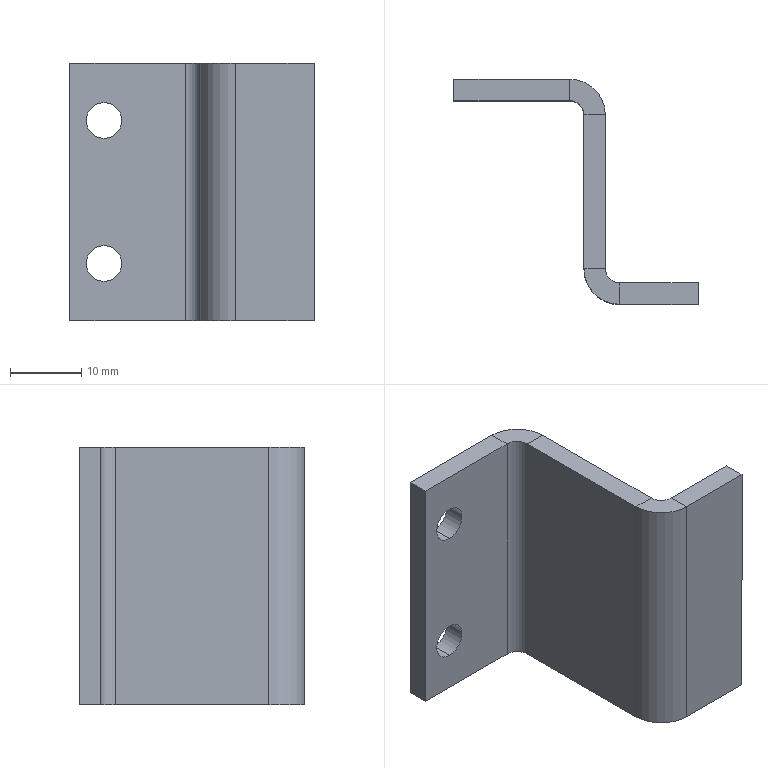Part | SolidWorks | features EdgeFlange 2, FlatPattern 1, HoleWzd 1, SMBaseFlange 1, SheetMetal 1 | 1 solid | 26 faces | box 34.18 x 31.5 x 36 mm | volume 6327 mm3 | plane 18 | cylinder 8 | commonest cylinder face diameters 5 x4 4 x2 10 x2
STEP:
#1=CARTESIAN_POINT('',(-21.41,25.5,-12.5));
#2=VERTEX_POINT('',#1);
#3=CARTESIAN_POINT('',(-21.41,25.5,-7.5));
#4=VERTEX_POINT('',#3);
#5=CARTESIAN_POINT('',(-21.41,25.5,-10.));
#6=DIRECTION('',(0.,1.,0.));
#7=DIRECTION('',(0.,0.,1.));
#8=AXIS2_PLACEMENT_3D('',#5,#6,#7);
#9=CIRCLE('',#8,2.5);
#10=EDGE_CURVE('',#2,#4,#9,.T.);
#11=ORIENTED_EDGE('',*,*,#10,.F.);
#12=CARTESIAN_POINT('',(-21.41,28.5,-12.5));
#13=VERTEX_POINT('',#12);
#14=CARTESIAN_POINT('',(-21.41,28.5,-12.5));
#15=DIRECTION('',(0.,1.,0.));
#16=VECTOR('',#15,1000.);
#17=LINE('',#14,#16);
#18=EDGE_CURVE('',#2,#13,#17,.T.);
#19=ORIENTED_EDGE('',*,*,#18,.T.);
#20=CARTESIAN_POINT('',(-21.41,28.5,-7.5));
#21=VERTEX_POINT('',#20);
#22=CARTESIAN_POINT('',(-21.41,28.5,-10.));
#23=DIRECTION('',(0.,1.,0.));
#24=DIRECTION('',(0.,0.,1.));
#25=AXIS2_PLACEMENT_3D('',#22,#23,#24);
#26=CIRCLE('',#25,2.5);
#27=EDGE_CURVE('',#13,#21,#26,.T.);
#28=ORIENTED_EDGE('',*,*,#27,.T.);
#29=CARTESIAN_POINT('',(-21.41,28.5,-7.5));
#30=DIRECTION('',(0.,1.,0.));
#31=VECTOR('',#30,1000.);
#32=LINE('',#29,#31);
#33=EDGE_CURVE('',#4,#21,#32,.T.);
#34=ORIENTED_EDGE('',*,*,#33,.F.);
#35=EDGE_LOOP('',(#11,#19,#28,#34));
#36=FACE_OUTER_BOUND('',#35,.T.);
#37=CARTESIAN_POINT('',(-21.41,28.5,-10.));
#38=DIRECTION('',(0.,1.,0.));
#39=DIRECTION('',(0.,0.,1.));
#40=AXIS2_PLACEMENT_3D('',#37,#38,#39);
#41=CYLINDRICAL_SURFACE('',#40,2.5);
#42=ADVANCED_FACE('',(#36),#41,.F.);
#43=CARTESIAN_POINT('',(-21.41,25.5,7.5));
#44=VERTEX_POINT('',#43);
#45=CARTESIAN_POINT('',(-21.41,25.5,12.5));
#46=VERTEX_POINT('',#45);
#47=CARTESIAN_POINT('',(-21.41,25.5,10.));
#48=DIRECTION('',(0.,1.,0.));
#49=DIRECTION('',(0.,0.,1.));
#50=AXIS2_PLACEMENT_3D('',#47,#48,#49);
#51=CIRCLE('',#50,2.5);
#52=EDGE_CURVE('',#44,#46,#51,.T.);
#53=ORIENTED_EDGE('',*,*,#52,.F.);
#54=CARTESIAN_POINT('',(-21.41,28.5,7.5));
#55=VERTEX_POINT('',#54);
#56=CARTESIAN_POINT('',(-21.41,28.5,7.5));
#57=DIRECTION('',(0.,1.,0.));
#58=VECTOR('',#57,1000.);
#59=LINE('',#56,#58);
#60=EDGE_CURVE('',#44,#55,#59,.T.);
#61=ORIENTED_EDGE('',*,*,#60,.T.);
#62=CARTESIAN_POINT('',(-21.41,28.5,12.5));
#63=VERTEX_POINT('',#62);
#64=CARTESIAN_POINT('',(-21.41,28.5,10.));
#65=DIRECTION('',(0.,1.,0.));
#66=DIRECTION('',(0.,0.,1.));
#67=AXIS2_PLACEMENT_3D('',#64,#65,#66);
#68=CIRCLE('',#67,2.5);
#69=EDGE_CURVE('',#55,#63,#68,.T.);
#70=ORIENTED_EDGE('',*,*,#69,.T.);
#71=CARTESIAN_POINT('',(-21.41,28.5,12.5));
#72=DIRECTION('',(0.,1.,0.));
#73=VECTOR('',#72,1000.);
#74=LINE('',#71,#73);
#75=EDGE_CURVE('',#46,#63,#74,.T.);
#76=ORIENTED_EDGE('',*,*,#75,.F.);
#77=EDGE_LOOP('',(#53,#61,#70,#76));
#78=FACE_OUTER_BOUND('',#77,.T.);
#79=CARTESIAN_POINT('',(-21.41,28.5,10.));
#80=DIRECTION('',(0.,1.,0.));
#81=DIRECTION('',(0.,0.,1.));
#82=AXIS2_PLACEMENT_3D('',#79,#80,#81);
#83=CYLINDRICAL_SURFACE('',#82,2.5);
#84=ADVANCED_FACE('',(#78),#83,.F.);
#85=CARTESIAN_POINT('',(-7.99,2.,-18.));
#86=VERTEX_POINT('',#85);
#87=CARTESIAN_POINT('',(-7.99,23.5,-18.));
#88=VERTEX_POINT('',#87);
#89=CARTESIAN_POINT('',(-7.99,28.5,-18.));
#90=DIRECTION('',(0.,1.,0.));
#91=VECTOR('',#90,1000.);
#92=LINE('',#89,#91);
#93=EDGE_CURVE('',#86,#88,#92,.T.);
#94=ORIENTED_EDGE('',*,*,#93,.T.);
#95=CARTESIAN_POINT('',(-4.99,23.5,-18.));
#96=VERTEX_POINT('',#95);
#97=CARTESIAN_POINT('',(-7.99,23.5,-18.));
#98=DIRECTION('',(1.,0.,0.));
#99=VECTOR('',#98,1000.);
#100=LINE('',#97,#99);
#101=EDGE_CURVE('',#88,#96,#100,.T.);
#102=ORIENTED_EDGE('',*,*,#101,.T.);
#103=CARTESIAN_POINT('',(-4.99,2.,-18.));
#104=VERTEX_POINT('',#103);
#105=CARTESIAN_POINT('',(-4.99,0.,-18.));
#106=DIRECTION('',(0.,1.,0.));
#107=VECTOR('',#106,1000.);
#108=LINE('',#105,#107);
#109=EDGE_CURVE('',#104,#96,#108,.T.);
#110=ORIENTED_EDGE('',*,*,#109,.F.);
#111=CARTESIAN_POINT('',(-7.99,2.,-18.));
#112=DIRECTION('',(-1.,0.,0.));
#113=VECTOR('',#112,1000.);
#114=LINE('',#111,#113);
#115=EDGE_CURVE('',#104,#86,#114,.T.);
#116=ORIENTED_EDGE('',*,*,#115,.T.);
#117=EDGE_LOOP('',(#94,#102,#110,#116));
#118=FACE_OUTER_BOUND('',#117,.T.);
#119=CARTESIAN_POINT('',(-7.99,28.5,-18.));
#120=DIRECTION('',(0.,0.,-1.));
#121=DIRECTION('',(-1.,0.,0.));
#122=AXIS2_PLACEMENT_3D('',#119,#120,#121);
#123=PLANE('',#122);
#124=ADVANCED_FACE('',(#118),#123,.T.);
#125=CARTESIAN_POINT('',(-7.99,23.5,18.));
#126=VERTEX_POINT('',#125);
#127=CARTESIAN_POINT('',(-7.99,2.,18.));
#128=VERTEX_POINT('',#127);
#129=CARTESIAN_POINT('',(-7.99,0.,18.));
#130=DIRECTION('',(0.,-1.,0.));
#131=VECTOR('',#130,1000.);
#132=LINE('',#129,#131);
#133=EDGE_CURVE('',#126,#128,#132,.T.);
#134=ORIENTED_EDGE('',*,*,#133,.F.);
#135=CARTESIAN_POINT('',(-7.99,23.5,-18.));
#136=DIRECTION('',(0.,0.,1.));
#137=VECTOR('',#136,1000.);
#138=LINE('',#135,#137);
#139=EDGE_CURVE('',#88,#126,#138,.T.);
#140=ORIENTED_EDGE('',*,*,#139,.F.);
#141=ORIENTED_EDGE('',*,*,#93,.F.);
#142=CARTESIAN_POINT('',(-7.99,2.,0.));
#143=DIRECTION('',(0.,0.,1.));
#144=VECTOR('',#143,1000.);
#145=LINE('',#142,#144);
#146=EDGE_CURVE('',#86,#128,#145,.T.);
#147=ORIENTED_EDGE('',*,*,#146,.T.);
#148=EDGE_LOOP('',(#134,#140,#141,#147));
#149=FACE_OUTER_BOUND('',#148,.T.);
#150=CARTESIAN_POINT('',(-7.99,0.,0.));
#151=DIRECTION('',(-1.,0.,0.));
#152=DIRECTION('',(0.,-1.,0.));
#153=AXIS2_PLACEMENT_3D('',#150,#151,#152);
#154=PLANE('',#153);
#155=ADVANCED_FACE('',(#149),#154,.T.);
#156=CARTESIAN_POINT('',(-4.99,23.5,18.));
#157=VERTEX_POINT('',#156);
#158=CARTESIAN_POINT('',(-4.99,23.5,-18.));
#159=DIRECTION('',(0.,0.,1.));
#160=VECTOR('',#159,1000.);
#161=LINE('',#158,#160);
#162=EDGE_CURVE('',#96,#157,#161,.T.);
#163=ORIENTED_EDGE('',*,*,#162,.T.);
#164=CARTESIAN_POINT('',(-4.99,2.,18.));
#165=VERTEX_POINT('',#164);
#166=CARTESIAN_POINT('',(-4.99,0.,18.));
#167=DIRECTION('',(0.,-1.,0.));
#168=VECTOR('',#167,1000.);
#169=LINE('',#166,#168);
#170=EDGE_CURVE('',#157,#165,#169,.T.);
#171=ORIENTED_EDGE('',*,*,#170,.T.);
#172=CARTESIAN_POINT('',(-4.99,2.,-18.));
#173=DIRECTION('',(0.,0.,1.));
#174=VECTOR('',#173,1000.);
#175=LINE('',#172,#174);
#176=EDGE_CURVE('',#104,#165,#175,.T.);
#177=ORIENTED_EDGE('',*,*,#176,.F.);
#178=ORIENTED_EDGE('',*,*,#109,.T.);
#179=EDGE_LOOP('',(#163,#171,#177,#178));
#180=FACE_OUTER_BOUND('',#179,.T.);
#181=CARTESIAN_POINT('',(-4.99,0.,0.));
#182=DIRECTION('',(-1.,0.,0.));
#183=DIRECTION('',(0.,-1.,0.));
#184=AXIS2_PLACEMENT_3D('',#181,#182,#183);
#185=PLANE('',#184);
#186=ADVANCED_FACE('',(#180),#185,.F.);
#187=CARTESIAN_POINT('',(-2.99,0.,18.));
#188=VERTEX_POINT('',#187);
#189=CARTESIAN_POINT('',(7.99,0.,18.));
#190=VERTEX_POINT('',#189);
#191=CARTESIAN_POINT('',(-7.99,0.,18.));
#192=DIRECTION('',(1.,0.,0.));
#193=VECTOR('',#192,1000.);
#194=LINE('',#191,#193);
#195=EDGE_CURVE('',#188,#190,#194,.T.);
#196=ORIENTED_EDGE('',*,*,#195,.F.);
#197=CARTESIAN_POINT('',(-2.99,-3.,18.));
#198=VERTEX_POINT('',#197);
#199=CARTESIAN_POINT('',(-2.99,0.,18.));
#200=DIRECTION('',(0.,-1.,0.));
#201=VECTOR('',#200,1000.);
#202=LINE('',#199,#201);
#203=EDGE_CURVE('',#188,#198,#202,.T.);
#204=ORIENTED_EDGE('',*,*,#203,.T.);
#205=CARTESIAN_POINT('',(7.99,-3.,18.));
#206=VERTEX_POINT('',#205);
#207=CARTESIAN_POINT('',(-7.99,-3.,18.));
#208=DIRECTION('',(1.,0.,0.));
#209=VECTOR('',#208,1000.);
#210=LINE('',#207,#209);
#211=EDGE_CURVE('',#198,#206,#210,.T.);
#212=ORIENTED_EDGE('',*,*,#211,.T.);
#213=CARTESIAN_POINT('',(7.99,-3.,18.));
#214=DIRECTION('',(0.,1.,0.));
#215=VECTOR('',#214,1000.);
#216=LINE('',#213,#215);
#217=EDGE_CURVE('',#206,#190,#216,.T.);
#218=ORIENTED_EDGE('',*,*,#217,.T.);
#219=EDGE_LOOP('',(#196,#204,#212,#218));
#220=FACE_OUTER_BOUND('',#219,.T.);
#221=CARTESIAN_POINT('',(-7.99,-3.,18.));
#222=DIRECTION('',(0.,0.,1.));
#223=DIRECTION('',(1.,0.,0.));
#224=AXIS2_PLACEMENT_3D('',#221,#222,#223);
#225=PLANE('',#224);
#226=ADVANCED_FACE('',(#220),#225,.T.);
#227=CARTESIAN_POINT('',(-2.99,-3.,-18.));
#228=VERTEX_POINT('',#227);
#229=CARTESIAN_POINT('',(-2.99,-3.,18.));
#230=DIRECTION('',(0.,0.,-1.));
#231=VECTOR('',#230,1000.);
#232=LINE('',#229,#231);
#233=EDGE_CURVE('',#198,#228,#232,.T.);
#234=ORIENTED_EDGE('',*,*,#233,.T.);
#235=CARTESIAN_POINT('',(7.99,-3.,-18.));
#236=VERTEX_POINT('',#235);
#237=CARTESIAN_POINT('',(-7.99,-3.,-18.));
#238=DIRECTION('',(-1.,0.,0.));
#239=VECTOR('',#238,1000.);
#240=LINE('',#237,#239);
#241=EDGE_CURVE('',#236,#228,#240,.T.);
#242=ORIENTED_EDGE('',*,*,#241,.F.);
#243=CARTESIAN_POINT('',(7.99,-3.,-18.));
#244=DIRECTION('',(0.,0.,-1.));
#245=VECTOR('',#244,1000.);
#246=LINE('',#243,#245);
#247=EDGE_CURVE('',#206,#236,#246,.T.);
#248=ORIENTED_EDGE('',*,*,#247,.F.);
#249=ORIENTED_EDGE('',*,*,#211,.F.);
#250=EDGE_LOOP('',(#234,#242,#248,#249));
#251=FACE_OUTER_BOUND('',#250,.T.);
#252=CARTESIAN_POINT('',(0.,-3.,0.));
#253=DIRECTION('',(0.,1.,0.));
#254=DIRECTION('',(0.,0.,1.));
#255=AXIS2_PLACEMENT_3D('',#252,#253,#254);
#256=PLANE('',#255);
#257=ADVANCED_FACE('',(#251),#256,.F.);
#258=CARTESIAN_POINT('',(7.99,0.,-18.));
#259=VERTEX_POINT('',#258);
#260=CARTESIAN_POINT('',(-2.99,0.,-18.));
#261=VERTEX_POINT('',#260);
#262=CARTESIAN_POINT('',(-7.99,0.,-18.));
#263=DIRECTION('',(-1.,0.,0.));
#264=VECTOR('',#263,1000.);
#265=LINE('',#262,#264);
#266=EDGE_CURVE('',#259,#261,#265,.T.);
#267=ORIENTED_EDGE('',*,*,#266,.T.);
#268=CARTESIAN_POINT('',(-2.99,0.,18.));
#269=DIRECTION('',(0.,0.,-1.));
#270=VECTOR('',#269,1000.);
#271=LINE('',#268,#270);
#272=EDGE_CURVE('',#188,#261,#271,.T.);
#273=ORIENTED_EDGE('',*,*,#272,.F.);
#274=ORIENTED_EDGE('',*,*,#195,.T.);
#275=CARTESIAN_POINT('',(7.99,0.,-18.));
#276=DIRECTION('',(0.,0.,-1.));
#277=VECTOR('',#276,1000.);
#278=LINE('',#275,#277);
#279=EDGE_CURVE('',#190,#259,#278,.T.);
#280=ORIENTED_EDGE('',*,*,#279,.T.);
#281=EDGE_LOOP('',(#267,#273,#274,#280));
#282=FACE_OUTER_BOUND('',#281,.T.);
#283=CARTESIAN_POINT('',(0.,0.,0.));
#284=DIRECTION('',(0.,1.,0.));
#285=DIRECTION('',(0.,0.,1.));
#286=AXIS2_PLACEMENT_3D('',#283,#284,#285);
#287=PLANE('',#286);
#288=ADVANCED_FACE('',(#282),#287,.T.);
#289=ORIENTED_EDGE('',*,*,#279,.F.);
#290=ORIENTED_EDGE('',*,*,#217,.F.);
#291=ORIENTED_EDGE('',*,*,#247,.T.);
#292=CARTESIAN_POINT('',(7.99,-3.,-18.));
#293=DIRECTION('',(0.,1.,0.));
#294=VECTOR('',#293,1000.);
#295=LINE('',#292,#294);
#296=EDGE_CURVE('',#236,#259,#295,.T.);
#297=ORIENTED_EDGE('',*,*,#296,.T.);
#298=EDGE_LOOP('',(#289,#290,#291,#297));
#299=FACE_OUTER_BOUND('',#298,.T.);
#300=CARTESIAN_POINT('',(7.99,-3.,-18.));
#301=DIRECTION('',(1.,0.,0.));
#302=DIRECTION('',(0.,0.,-1.));
#303=AXIS2_PLACEMENT_3D('',#300,#301,#302);
#304=PLANE('',#303);
#305=ADVANCED_FACE('',(#299),#304,.T.);
#306=CARTESIAN_POINT('',(-2.99,0.,-18.));
#307=DIRECTION('',(0.,-1.,0.));
#308=VECTOR('',#307,1000.);
#309=LINE('',#306,#308);
#310=EDGE_CURVE('',#261,#228,#309,.T.);
#311=ORIENTED_EDGE('',*,*,#310,.F.);
#312=ORIENTED_EDGE('',*,*,#266,.F.);
#313=ORIENTED_EDGE('',*,*,#296,.F.);
#314=ORIENTED_EDGE('',*,*,#241,.T.);
#315=EDGE_LOOP('',(#311,#312,#313,#314));
#316=FACE_OUTER_BOUND('',#315,.T.);
#317=CARTESIAN_POINT('',(-7.99,-3.,-18.));
#318=DIRECTION('',(0.,0.,-1.));
#319=DIRECTION('',(-1.,0.,0.));
#320=AXIS2_PLACEMENT_3D('',#317,#318,#319);
#321=PLANE('',#320);
#322=ADVANCED_FACE('',(#316),#321,.T.);
#323=ORIENTED_EDGE('',*,*,#115,.F.);
#324=CARTESIAN_POINT('',(-2.99,2.,-18.));
#325=DIRECTION('',(0.,0.,-1.));
#326=DIRECTION('',(1.,0.,0.));
#327=AXIS2_PLACEMENT_3D('',#324,#325,#326);
#328=CIRCLE('',#327,2.);
#329=EDGE_CURVE('',#261,#104,#328,.T.);
#330=ORIENTED_EDGE('',*,*,#329,.F.);
#331=ORIENTED_EDGE('',*,*,#310,.T.);
#332=CARTESIAN_POINT('',(-2.99,2.,-18.));
#333=DIRECTION('',(0.,0.,-1.));
#334=DIRECTION('',(1.,0.,0.));
#335=AXIS2_PLACEMENT_3D('',#332,#333,#334);
#336=CIRCLE('',#335,5.);
#337=EDGE_CURVE('',#228,#86,#336,.T.);
#338=ORIENTED_EDGE('',*,*,#337,.T.);
#339=EDGE_LOOP('',(#323,#330,#331,#338));
#340=FACE_OUTER_BOUND('',#339,.T.);
#341=CARTESIAN_POINT('',(-2.99,2.,-18.));
#342=DIRECTION('',(0.,0.,-1.));
#343=DIRECTION('',(-1.,0.,0.));
#344=AXIS2_PLACEMENT_3D('',#341,#342,#343);
#345=PLANE('',#344);
#346=ADVANCED_FACE('',(#340),#345,.T.);
#347=CARTESIAN_POINT('',(-2.99,2.,18.));
#348=DIRECTION('',(0.,0.,1.));
#349=DIRECTION('',(1.,0.,0.));
#350=AXIS2_PLACEMENT_3D('',#347,#348,#349);
#351=CIRCLE('',#350,2.);
#352=EDGE_CURVE('',#165,#188,#351,.T.);
#353=ORIENTED_EDGE('',*,*,#352,.F.);
#354=CARTESIAN_POINT('',(-4.99,2.,18.));
#355=DIRECTION('',(-1.,0.,0.));
#356=VECTOR('',#355,1000.);
#357=LINE('',#354,#356);
#358=EDGE_CURVE('',#165,#128,#357,.T.);
#359=ORIENTED_EDGE('',*,*,#358,.T.);
#360=CARTESIAN_POINT('',(-2.99,2.,18.));
#361=DIRECTION('',(0.,0.,1.));
#362=DIRECTION('',(1.,0.,0.));
#363=AXIS2_PLACEMENT_3D('',#360,#361,#362);
#364=CIRCLE('',#363,5.);
#365=EDGE_CURVE('',#128,#198,#364,.T.);
#366=ORIENTED_EDGE('',*,*,#365,.T.);
#367=ORIENTED_EDGE('',*,*,#203,.F.);
#368=EDGE_LOOP('',(#353,#359,#366,#367));
#369=FACE_OUTER_BOUND('',#368,.T.);
#370=CARTESIAN_POINT('',(-2.99,2.,18.));
#371=DIRECTION('',(0.,0.,-1.));
#372=DIRECTION('',(-1.,0.,0.));
#373=AXIS2_PLACEMENT_3D('',#370,#371,#372);
#374=PLANE('',#373);
#375=ADVANCED_FACE('',(#369),#374,.F.);
#376=ORIENTED_EDGE('',*,*,#233,.F.);
#377=ORIENTED_EDGE('',*,*,#365,.F.);
#378=ORIENTED_EDGE('',*,*,#146,.F.);
#379=ORIENTED_EDGE('',*,*,#337,.F.);
#380=EDGE_LOOP('',(#376,#377,#378,#379));
#381=FACE_OUTER_BOUND('',#380,.T.);
#382=CARTESIAN_POINT('',(-2.99,2.,18.));
#383=DIRECTION('',(0.,0.,1.));
#384=DIRECTION('',(-1.,0.,0.));
#385=AXIS2_PLACEMENT_3D('',#382,#383,#384);
#386=CYLINDRICAL_SURFACE('',#385,5.);
#387=ADVANCED_FACE('',(#381),#386,.T.);
#388=ORIENTED_EDGE('',*,*,#272,.T.);
#389=ORIENTED_EDGE('',*,*,#329,.T.);
#390=ORIENTED_EDGE('',*,*,#176,.T.);
#391=ORIENTED_EDGE('',*,*,#352,.T.);
#392=EDGE_LOOP('',(#388,#389,#390,#391));
#393=FACE_OUTER_BOUND('',#392,.T.);
#394=CARTESIAN_POINT('',(-2.99,2.,18.));
#395=DIRECTION('',(0.,0.,1.));
#396=DIRECTION('',(-1.,0.,0.));
#397=AXIS2_PLACEMENT_3D('',#394,#395,#396);
#398=CYLINDRICAL_SURFACE('',#397,2.);
#399=ADVANCED_FACE('',(#393),#398,.F.);
#400=CARTESIAN_POINT('',(-7.99,23.5,18.));
#401=DIRECTION('',(1.,0.,0.));
#402=VECTOR('',#401,1000.);
#403=LINE('',#400,#402);
#404=EDGE_CURVE('',#126,#157,#403,.T.);
#405=ORIENTED_EDGE('',*,*,#404,.F.);
#406=ORIENTED_EDGE('',*,*,#133,.T.);
#407=ORIENTED_EDGE('',*,*,#358,.F.);
#408=ORIENTED_EDGE('',*,*,#170,.F.);
#409=EDGE_LOOP('',(#405,#406,#407,#408));
#410=FACE_OUTER_BOUND('',#409,.T.);
#411=CARTESIAN_POINT('',(-7.99,0.,18.));
#412=DIRECTION('',(0.,0.,1.));
#413=DIRECTION('',(1.,0.,0.));
#414=AXIS2_PLACEMENT_3D('',#411,#412,#413);
#415=PLANE('',#414);
#416=ADVANCED_FACE('',(#410),#415,.T.);
#417=CARTESIAN_POINT('',(-9.99,25.5,18.));
#418=VERTEX_POINT('',#417);
#419=CARTESIAN_POINT('',(-9.99,28.5,18.));
#420=VERTEX_POINT('',#419);
#421=CARTESIAN_POINT('',(-9.99,28.5,18.));
#422=DIRECTION('',(0.,1.,0.));
#423=VECTOR('',#422,1000.);
#424=LINE('',#421,#423);
#425=EDGE_CURVE('',#418,#420,#424,.T.);
#426=ORIENTED_EDGE('',*,*,#425,.F.);
#427=CARTESIAN_POINT('',(-9.99,23.5,18.));
#428=DIRECTION('',(0.,0.,1.));
#429=DIRECTION('',(-1.,0.,0.));
#430=AXIS2_PLACEMENT_3D('',#427,#428,#429);
#431=CIRCLE('',#430,2.);
#432=EDGE_CURVE('',#126,#418,#431,.T.);
#433=ORIENTED_EDGE('',*,*,#432,.F.);
#434=ORIENTED_EDGE('',*,*,#404,.T.);
#435=CARTESIAN_POINT('',(-9.99,23.5,18.));
#436=DIRECTION('',(0.,0.,1.));
#437=DIRECTION('',(-1.,0.,0.));
#438=AXIS2_PLACEMENT_3D('',#435,#436,#437);
#439=CIRCLE('',#438,5.);
#440=EDGE_CURVE('',#157,#420,#439,.T.);
#441=ORIENTED_EDGE('',*,*,#440,.T.);
#442=EDGE_LOOP('',(#426,#433,#434,#441));
#443=FACE_OUTER_BOUND('',#442,.T.);
#444=CARTESIAN_POINT('',(-9.99,23.5,18.));
#445=DIRECTION('',(0.,0.,1.));
#446=DIRECTION('',(1.,0.,0.));
#447=AXIS2_PLACEMENT_3D('',#444,#445,#446);
#448=PLANE('',#447);
#449=ADVANCED_FACE('',(#443),#448,.T.);
#450=CARTESIAN_POINT('',(-9.99,25.5,-18.));
#451=VERTEX_POINT('',#450);
#452=CARTESIAN_POINT('',(-9.99,23.5,-18.));
#453=DIRECTION('',(0.,0.,-1.));
#454=DIRECTION('',(-1.,0.,0.));
#455=AXIS2_PLACEMENT_3D('',#452,#453,#454);
#456=CIRCLE('',#455,2.);
#457=EDGE_CURVE('',#451,#88,#456,.T.);
#458=ORIENTED_EDGE('',*,*,#457,.F.);
#459=CARTESIAN_POINT('',(-9.99,28.5,-18.));
#460=VERTEX_POINT('',#459);
#461=CARTESIAN_POINT('',(-9.99,25.5,-18.));
#462=DIRECTION('',(0.,1.,0.));
#463=VECTOR('',#462,1000.);
#464=LINE('',#461,#463);
#465=EDGE_CURVE('',#451,#460,#464,.T.);
#466=ORIENTED_EDGE('',*,*,#465,.T.);
#467=CARTESIAN_POINT('',(-9.99,23.5,-18.));
#468=DIRECTION('',(0.,0.,-1.));
#469=DIRECTION('',(-1.,0.,0.));
#470=AXIS2_PLACEMENT_3D('',#467,#468,#469);
#471=CIRCLE('',#470,5.);
#472=EDGE_CURVE('',#460,#96,#471,.T.);
#473=ORIENTED_EDGE('',*,*,#472,.T.);
#474=ORIENTED_EDGE('',*,*,#101,.F.);
#475=EDGE_LOOP('',(#458,#466,#473,#474));
#476=FACE_OUTER_BOUND('',#475,.T.);
#477=CARTESIAN_POINT('',(-9.99,23.5,-18.));
#478=DIRECTION('',(0.,0.,1.));
#479=DIRECTION('',(1.,0.,0.));
#480=AXIS2_PLACEMENT_3D('',#477,#478,#479);
#481=PLANE('',#480);
#482=ADVANCED_FACE('',(#476),#481,.F.);
#483=ORIENTED_EDGE('',*,*,#162,.F.);
#484=ORIENTED_EDGE('',*,*,#472,.F.);
#485=CARTESIAN_POINT('',(-9.99,28.5,0.));
#486=DIRECTION('',(0.,0.,-1.));
#487=VECTOR('',#486,1000.);
#488=LINE('',#485,#487);
#489=EDGE_CURVE('',#420,#460,#488,.T.);
#490=ORIENTED_EDGE('',*,*,#489,.F.);
#491=ORIENTED_EDGE('',*,*,#440,.F.);
#492=EDGE_LOOP('',(#483,#484,#490,#491));
#493=FACE_OUTER_BOUND('',#492,.T.);
#494=CARTESIAN_POINT('',(-9.99,23.5,-18.));
#495=DIRECTION('',(0.,0.,-1.));
#496=DIRECTION('',(0.,1.,0.));
#497=AXIS2_PLACEMENT_3D('',#494,#495,#496);
#498=CYLINDRICAL_SURFACE('',#497,5.);
#499=ADVANCED_FACE('',(#493),#498,.T.);
#500=ORIENTED_EDGE('',*,*,#139,.T.);
#501=ORIENTED_EDGE('',*,*,#432,.T.);
#502=CARTESIAN_POINT('',(-9.99,25.5,18.));
#503=DIRECTION('',(0.,0.,-1.));
#504=VECTOR('',#503,1000.);
#505=LINE('',#502,#504);
#506=EDGE_CURVE('',#418,#451,#505,.T.);
#507=ORIENTED_EDGE('',*,*,#506,.T.);
#508=ORIENTED_EDGE('',*,*,#457,.T.);
#509=EDGE_LOOP('',(#500,#501,#507,#508));
#510=FACE_OUTER_BOUND('',#509,.T.);
#511=CARTESIAN_POINT('',(-9.99,23.5,-18.));
#512=DIRECTION('',(0.,0.,-1.));
#513=DIRECTION('',(0.,1.,0.));
#514=AXIS2_PLACEMENT_3D('',#511,#512,#513);
#515=CYLINDRICAL_SURFACE('',#514,2.);
#516=ADVANCED_FACE('',(#510),#515,.F.);
#517=CARTESIAN_POINT('',(-26.19,28.5,-18.));
#518=VERTEX_POINT('',#517);
#519=CARTESIAN_POINT('',(-7.99,28.5,-18.));
#520=DIRECTION('',(1.,0.,0.));
#521=VECTOR('',#520,1000.);
#522=LINE('',#519,#521);
#523=EDGE_CURVE('',#518,#460,#522,.T.);
#524=ORIENTED_EDGE('',*,*,#523,.T.);
#525=ORIENTED_EDGE('',*,*,#465,.F.);
#526=CARTESIAN_POINT('',(-26.19,25.5,-18.));
#527=VERTEX_POINT('',#526);
#528=CARTESIAN_POINT('',(0.,25.5,-18.));
#529=DIRECTION('',(1.,0.,0.));
#530=VECTOR('',#529,1000.);
#531=LINE('',#528,#530);
#532=EDGE_CURVE('',#527,#451,#531,.T.);
#533=ORIENTED_EDGE('',*,*,#532,.F.);
#534=CARTESIAN_POINT('',(-26.19,28.5,-18.));
#535=DIRECTION('',(0.,-1.,0.));
#536=VECTOR('',#535,1000.);
#537=LINE('',#534,#536);
#538=EDGE_CURVE('',#518,#527,#537,.T.);
#539=ORIENTED_EDGE('',*,*,#538,.F.);
#540=EDGE_LOOP('',(#524,#525,#533,#539));
#541=FACE_OUTER_BOUND('',#540,.T.);
#542=CARTESIAN_POINT('',(-7.99,28.5,-18.));
#543=DIRECTION('',(0.,0.,-1.));
#544=DIRECTION('',(-1.,0.,0.));
#545=AXIS2_PLACEMENT_3D('',#542,#543,#544);
#546=PLANE('',#545);
#547=ADVANCED_FACE('',(#541),#546,.T.);
#548=CARTESIAN_POINT('',(-26.19,25.5,18.));
#549=VERTEX_POINT('',#548);
#550=CARTESIAN_POINT('',(0.,25.5,18.));
#551=DIRECTION('',(-1.,0.,0.));
#552=VECTOR('',#551,1000.);
#553=LINE('',#550,#552);
#554=EDGE_CURVE('',#418,#549,#553,.T.);
#555=ORIENTED_EDGE('',*,*,#554,.F.);
#556=ORIENTED_EDGE('',*,*,#425,.T.);
#557=CARTESIAN_POINT('',(-26.19,28.5,18.));
#558=VERTEX_POINT('',#557);
#559=CARTESIAN_POINT('',(-26.19,28.5,18.));
#560=DIRECTION('',(-1.,0.,0.));
#561=VECTOR('',#560,1000.);
#562=LINE('',#559,#561);
#563=EDGE_CURVE('',#420,#558,#562,.T.);
#564=ORIENTED_EDGE('',*,*,#563,.T.);
#565=CARTESIAN_POINT('',(-26.19,28.5,18.));
#566=DIRECTION('',(0.,-1.,0.));
#567=VECTOR('',#566,1000.);
#568=LINE('',#565,#567);
#569=EDGE_CURVE('',#558,#549,#568,.T.);
#570=ORIENTED_EDGE('',*,*,#569,.T.);
#571=EDGE_LOOP('',(#555,#556,#564,#570));
#572=FACE_OUTER_BOUND('',#571,.T.);
#573=CARTESIAN_POINT('',(-26.19,28.5,18.));
#574=DIRECTION('',(0.,0.,1.));
#575=DIRECTION('',(1.,0.,0.));
#576=AXIS2_PLACEMENT_3D('',#573,#574,#575);
#577=PLANE('',#576);
#578=ADVANCED_FACE('',(#572),#577,.T.);
#579=CARTESIAN_POINT('',(-21.41,28.5,-10.));
#580=DIRECTION('',(0.,1.,0.));
#581=DIRECTION('',(0.,0.,1.));
#582=AXIS2_PLACEMENT_3D('',#579,#580,#581);
#583=CIRCLE('',#582,2.5);
#584=EDGE_CURVE('',#21,#13,#583,.T.);
#585=ORIENTED_EDGE('',*,*,#584,.F.);
#586=ORIENTED_EDGE('',*,*,#27,.F.);
#587=EDGE_LOOP('',(#585,#586));
#588=FACE_BOUND('',#587,.T.);
#589=CARTESIAN_POINT('',(-21.41,28.5,10.));
#590=DIRECTION('',(0.,1.,0.));
#591=DIRECTION('',(0.,0.,1.));
#592=AXIS2_PLACEMENT_3D('',#589,#590,#591);
#593=CIRCLE('',#592,2.5);
#594=EDGE_CURVE('',#63,#55,#593,.T.);
#595=ORIENTED_EDGE('',*,*,#594,.F.);
#596=ORIENTED_EDGE('',*,*,#69,.F.);
#597=EDGE_LOOP('',(#595,#596));
#598=FACE_BOUND('',#597,.T.);
#599=ORIENTED_EDGE('',*,*,#563,.F.);
#600=ORIENTED_EDGE('',*,*,#489,.T.);
#601=ORIENTED_EDGE('',*,*,#523,.F.);
#602=CARTESIAN_POINT('',(-26.19,28.5,-18.));
#603=DIRECTION('',(0.,0.,-1.));
#604=VECTOR('',#603,1000.);
#605=LINE('',#602,#604);
#606=EDGE_CURVE('',#558,#518,#605,.T.);
#607=ORIENTED_EDGE('',*,*,#606,.F.);
#608=EDGE_LOOP('',(#599,#600,#601,#607));
#609=FACE_OUTER_BOUND('',#608,.T.);
#610=CARTESIAN_POINT('',(0.,28.5,0.));
#611=DIRECTION('',(0.,1.,0.));
#612=DIRECTION('',(0.,0.,1.));
#613=AXIS2_PLACEMENT_3D('',#610,#611,#612);
#614=PLANE('',#613);
#615=ADVANCED_FACE('',(#588,#598,#609),#614,.T.);
#616=CARTESIAN_POINT('',(-21.41,25.5,-10.));
#617=DIRECTION('',(0.,1.,0.));
#618=DIRECTION('',(0.,0.,1.));
#619=AXIS2_PLACEMENT_3D('',#616,#617,#618);
#620=CIRCLE('',#619,2.5);
#621=EDGE_CURVE('',#4,#2,#620,.T.);
#622=ORIENTED_EDGE('',*,*,#621,.T.);
#623=ORIENTED_EDGE('',*,*,#10,.T.);
#624=EDGE_LOOP('',(#622,#623));
#625=FACE_BOUND('',#624,.T.);
#626=CARTESIAN_POINT('',(-21.41,25.5,10.));
#627=DIRECTION('',(0.,1.,0.));
#628=DIRECTION('',(0.,0.,1.));
#629=AXIS2_PLACEMENT_3D('',#626,#627,#628);
#630=CIRCLE('',#629,2.5);
#631=EDGE_CURVE('',#46,#44,#630,.T.);
#632=ORIENTED_EDGE('',*,*,#631,.T.);
#633=ORIENTED_EDGE('',*,*,#52,.T.);
#634=EDGE_LOOP('',(#632,#633));
#635=FACE_BOUND('',#634,.T.);
#636=ORIENTED_EDGE('',*,*,#506,.F.);
#637=ORIENTED_EDGE('',*,*,#554,.T.);
#638=CARTESIAN_POINT('',(-26.19,25.5,0.));
#639=DIRECTION('',(0.,0.,-1.));
#640=VECTOR('',#639,1000.);
#641=LINE('',#638,#640);
#642=EDGE_CURVE('',#549,#527,#641,.T.);
#643=ORIENTED_EDGE('',*,*,#642,.T.);
#644=ORIENTED_EDGE('',*,*,#532,.T.);
#645=EDGE_LOOP('',(#636,#637,#643,#644));
#646=FACE_OUTER_BOUND('',#645,.T.);
#647=CARTESIAN_POINT('',(0.,25.5,0.));
#648=DIRECTION('',(0.,1.,0.));
#649=DIRECTION('',(0.,0.,1.));
#650=AXIS2_PLACEMENT_3D('',#647,#648,#649);
#651=PLANE('',#650);
#652=ADVANCED_FACE('',(#625,#635,#646),#651,.F.);
#653=ORIENTED_EDGE('',*,*,#642,.F.);
#654=ORIENTED_EDGE('',*,*,#569,.F.);
#655=ORIENTED_EDGE('',*,*,#606,.T.);
#656=ORIENTED_EDGE('',*,*,#538,.T.);
#657=EDGE_LOOP('',(#653,#654,#655,#656));
#658=FACE_OUTER_BOUND('',#657,.T.);
#659=CARTESIAN_POINT('',(-26.19,28.5,-18.));
#660=DIRECTION('',(-1.,0.,0.));
#661=DIRECTION('',(0.,-1.,0.));
#662=AXIS2_PLACEMENT_3D('',#659,#660,#661);
#663=PLANE('',#662);
#664=ADVANCED_FACE('',(#658),#663,.T.);
#665=ORIENTED_EDGE('',*,*,#60,.F.);
#666=ORIENTED_EDGE('',*,*,#631,.F.);
#667=ORIENTED_EDGE('',*,*,#75,.T.);
#668=ORIENTED_EDGE('',*,*,#594,.T.);
#669=EDGE_LOOP('',(#665,#666,#667,#668));
#670=FACE_OUTER_BOUND('',#669,.T.);
#671=CARTESIAN_POINT('',(-21.41,28.5,10.));
#672=DIRECTION('',(0.,1.,0.));
#673=DIRECTION('',(0.,0.,1.));
#674=AXIS2_PLACEMENT_3D('',#671,#672,#673);
#675=CYLINDRICAL_SURFACE('',#674,2.5);
#676=ADVANCED_FACE('',(#670),#675,.F.);
#677=ORIENTED_EDGE('',*,*,#18,.F.);
#678=ORIENTED_EDGE('',*,*,#621,.F.);
#679=ORIENTED_EDGE('',*,*,#33,.T.);
#680=ORIENTED_EDGE('',*,*,#584,.T.);
#681=EDGE_LOOP('',(#677,#678,#679,#680));
#682=FACE_OUTER_BOUND('',#681,.T.);
#683=CARTESIAN_POINT('',(-21.41,28.5,-10.));
#684=DIRECTION('',(0.,1.,0.));
#685=DIRECTION('',(0.,0.,1.));
#686=AXIS2_PLACEMENT_3D('',#683,#684,#685);
#687=CYLINDRICAL_SURFACE('',#686,2.5);
#688=ADVANCED_FACE('',(#682),#687,.F.);
#689=CLOSED_SHELL('',(#42,#84,#124,#155,#186,#226,#257,#288,#305,#322,#346,#375,#387,#399,#416,#449,#482,#499,#516,#547,#578,#615,#652,#664,#676,#688));
#690=MANIFOLD_SOLID_BREP('',#689);
#691=CARTESIAN_POINT('',(0.,0.,0.));
#692=DIRECTION('',(0.,0.,1.));
#693=DIRECTION('',(1.,0.,0.));
#694=AXIS2_PLACEMENT_3D('',#691,#692,#693);
#695=(LENGTH_UNIT()NAMED_UNIT(*)SI_UNIT(.MILLI.,.METRE.));
#696=UNCERTAINTY_MEASURE_WITH_UNIT(LENGTH_MEASURE(0.00001),#695,'','');
#697=(NAMED_UNIT(*)PLANE_ANGLE_UNIT()SI_UNIT($,.RADIAN.));
#698=(NAMED_UNIT(*)SI_UNIT($,.STERADIAN.)SOLID_ANGLE_UNIT());
#699=(GEOMETRIC_REPRESENTATION_CONTEXT(3)GLOBAL_UNCERTAINTY_ASSIGNED_CONTEXT((#696))GLOBAL_UNIT_ASSIGNED_CONTEXT((#695,#697,#698))REPRESENTATION_CONTEXT('',''));
#700=ADVANCED_BREP_SHAPE_REPRESENTATION('',(#690,#694),#699);